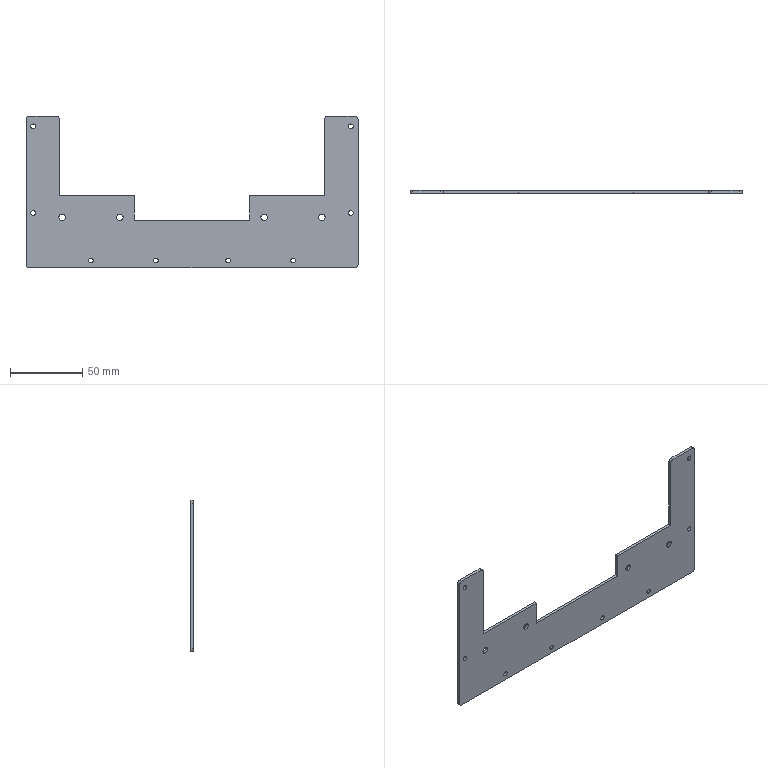Part | STEP file | 1 solid | 44 faces | box 230 x 2 x 105 mm | volume 25066 mm3 | cylinder 30 | plane 14 | commonest cylinder face diameters 3.3 x16 4.5 x8 4 x6